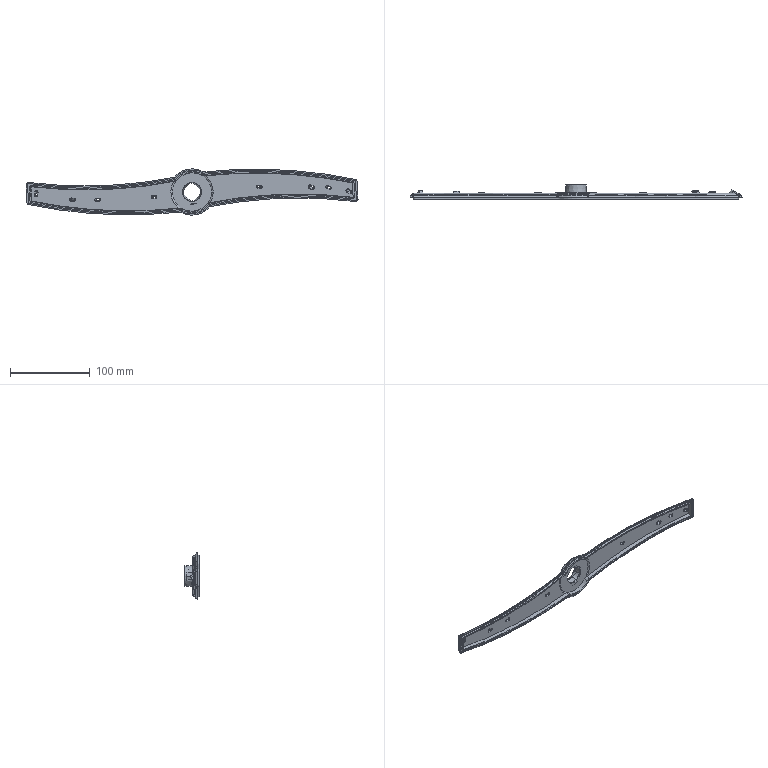Part | STEP file | MSBR-28 | 1 solid | 502 faces | box 415.551 x 17.694 x 58 mm | volume 32768 mm3 | cylinder 196 | spline 95 | plane 88 | torus 86 | sphere 29 | cone 8 | commonest cylinder face diameters 1 x70 2 x55 4 x11 0.6 x7 6 x6 0.4 x4